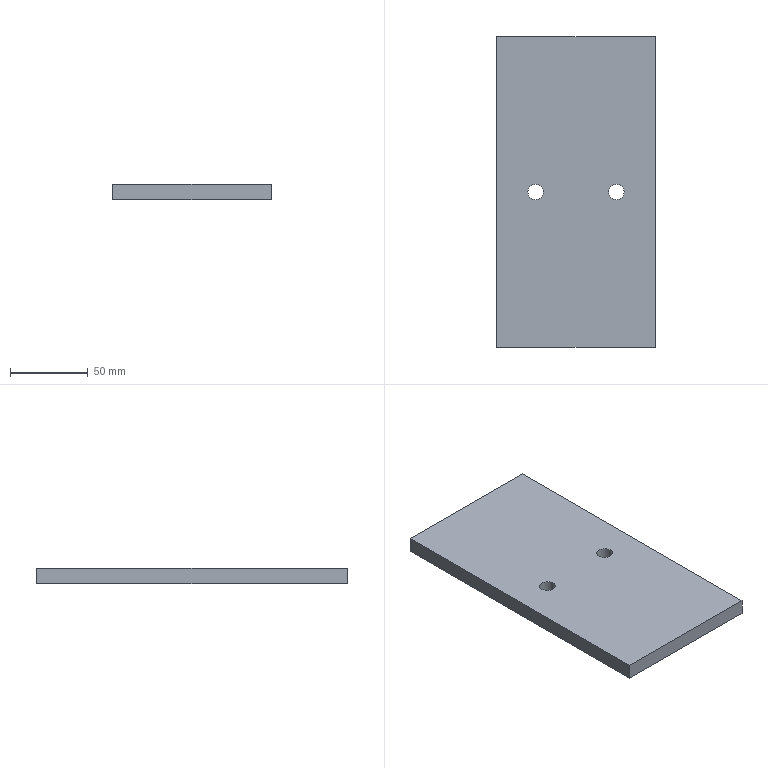Part | STEP file | E3-导轨限位Plate | 1 solid | 10 faces | box 102 x 200 x 10 mm | volume 202429 mm3 | plane 6 | cylinder 4 | commonest cylinder face diameters 10 x4
STEP:
#1=CARTESIAN_POINT('',(0.,0.,0.));
#2=DIRECTION('',(0.,0.,1.));
#3=DIRECTION('',(1.,0.,0.));
#4=AXIS2_PLACEMENT_3D('',#1,#2,#3);
#5=CARTESIAN_POINT('',(-21.,0.,0.));
#6=VERTEX_POINT('',#5);
#7=CARTESIAN_POINT('',(-21.,0.,-10.));
#8=VERTEX_POINT('',#7);
#9=CARTESIAN_POINT('',(-21.,0.,-10.));
#10=DIRECTION('',(0.,0.,-1.));
#11=VECTOR('',#10,1.);
#12=LINE('',#9,#11);
#13=CARTESIAN_POINT('',(-26.,0.,-10.));
#14=DIRECTION('',(0.,0.,-1.));
#15=DIRECTION('',(1.,0.,0.));
#16=AXIS2_PLACEMENT_3D('',#13,#14,#15);
#17=CYLINDRICAL_SURFACE('',#16,5.);
#18=CARTESIAN_POINT('',(6.283,0.));
#19=DIRECTION('',(0.,1.));
#20=VECTOR('',#19,1.);
#21=LINE('',#18,#20);
#22=(GEOMETRIC_REPRESENTATION_CONTEXT(2)PARAMETRIC_REPRESENTATION_CONTEXT()REPRESENTATION_CONTEXT('',''));
#23=DEFINITIONAL_REPRESENTATION('',(#21),#22);
#24=PCURVE('',#17,#23);
#25=CARTESIAN_POINT('',(-26.,0.,-10.));
#26=DIRECTION('',(0.,0.,-1.));
#27=DIRECTION('',(1.,0.,0.));
#28=AXIS2_PLACEMENT_3D('',#25,#26,#27);
#29=CYLINDRICAL_SURFACE('',#28,5.);
#30=CARTESIAN_POINT('',(0.,0.));
#31=DIRECTION('',(0.,1.));
#32=VECTOR('',#31,1.);
#33=LINE('',#30,#32);
#34=(GEOMETRIC_REPRESENTATION_CONTEXT(2)PARAMETRIC_REPRESENTATION_CONTEXT()REPRESENTATION_CONTEXT('',''));
#35=DEFINITIONAL_REPRESENTATION('',(#33),#34);
#36=PCURVE('',#29,#35);
#37=SURFACE_CURVE('',#12,(#24,#36),.PCURVE_S1.);
#38=EDGE_CURVE('',#6,#8,#37,.T.);
#39=ORIENTED_EDGE('',*,*,#38,.T.);
#40=CARTESIAN_POINT('',(-31.,0.,-10.));
#41=VERTEX_POINT('',#40);
#42=CARTESIAN_POINT('',(-26.,0.,-10.));
#43=DIRECTION('',(0.,0.,1.));
#44=DIRECTION('',(1.,0.,0.));
#45=AXIS2_PLACEMENT_3D('',#42,#43,#44);
#46=CIRCLE('',#45,5.);
#47=CARTESIAN_POINT('',(6.283,0.));
#48=DIRECTION('',(-1.,0.));
#49=VECTOR('',#48,1.);
#50=LINE('',#47,#49);
#51=(GEOMETRIC_REPRESENTATION_CONTEXT(2)PARAMETRIC_REPRESENTATION_CONTEXT()REPRESENTATION_CONTEXT('',''));
#52=DEFINITIONAL_REPRESENTATION('',(#50),#51);
#53=PCURVE('',#17,#52);
#54=CARTESIAN_POINT('',(0.,0.,-10.));
#55=DIRECTION('',(0.,0.,-1.));
#56=DIRECTION('',(1.,0.,0.));
#57=AXIS2_PLACEMENT_3D('',#54,#55,#56);
#58=PLANE('',#57);
#59=CARTESIAN_POINT('',(-21.,0.));
#60=CARTESIAN_POINT('',(-21.,-8.66));
#61=CARTESIAN_POINT('',(-28.5,-4.33));
#62=CARTESIAN_POINT('',(-36.,0.));
#63=CARTESIAN_POINT('',(-28.5,4.33));
#64=CARTESIAN_POINT('',(-21.,8.66));
#65=CARTESIAN_POINT('',(-21.,0.));
#66=(BOUNDED_CURVE()B_SPLINE_CURVE(2,(#59,#60,#61,#62,#63,#64,#65),.UNSPECIFIED.,.T.,.F.)B_SPLINE_CURVE_WITH_KNOTS((1,2,2,2,2,1),(-2.094,0.,2.094,4.189,6.283,8.378),.UNSPECIFIED.)CURVE()GEOMETRIC_REPRESENTATION_ITEM()RATIONAL_B_SPLINE_CURVE((1.,0.5,1.,0.5,1.,0.5,1.))REPRESENTATION_ITEM(''));
#67=(GEOMETRIC_REPRESENTATION_CONTEXT(2)PARAMETRIC_REPRESENTATION_CONTEXT()REPRESENTATION_CONTEXT('',''));
#68=DEFINITIONAL_REPRESENTATION('',(#66),#67);
#69=PCURVE('',#58,#68);
#70=SURFACE_CURVE('',#46,(#53,#69),.PCURVE_S1.);
#71=EDGE_CURVE('',#8,#41,#70,.T.);
#72=ORIENTED_EDGE('',*,*,#71,.T.);
#73=CARTESIAN_POINT('',(-31.,0.,0.));
#74=VERTEX_POINT('',#73);
#75=CARTESIAN_POINT('',(-31.,0.,-10.));
#76=DIRECTION('',(0.,0.,-1.));
#77=VECTOR('',#76,1.);
#78=LINE('',#75,#77);
#79=CARTESIAN_POINT('',(3.142,0.));
#80=DIRECTION('',(0.,1.));
#81=VECTOR('',#80,1.);
#82=LINE('',#79,#81);
#83=(GEOMETRIC_REPRESENTATION_CONTEXT(2)PARAMETRIC_REPRESENTATION_CONTEXT()REPRESENTATION_CONTEXT('',''));
#84=DEFINITIONAL_REPRESENTATION('',(#82),#83);
#85=PCURVE('',#17,#84);
#86=CARTESIAN_POINT('',(3.142,0.));
#87=DIRECTION('',(0.,1.));
#88=VECTOR('',#87,1.);
#89=LINE('',#86,#88);
#90=(GEOMETRIC_REPRESENTATION_CONTEXT(2)PARAMETRIC_REPRESENTATION_CONTEXT()REPRESENTATION_CONTEXT('',''));
#91=DEFINITIONAL_REPRESENTATION('',(#89),#90);
#92=PCURVE('',#29,#91);
#93=SURFACE_CURVE('',#78,(#85,#92),.PCURVE_S1.);
#94=EDGE_CURVE('',#74,#41,#93,.T.);
#95=ORIENTED_EDGE('',*,*,#94,.F.);
#96=CARTESIAN_POINT('',(-26.,0.,0.));
#97=DIRECTION('',(0.,0.,1.));
#98=DIRECTION('',(1.,0.,0.));
#99=AXIS2_PLACEMENT_3D('',#96,#97,#98);
#100=CIRCLE('',#99,5.);
#101=CARTESIAN_POINT('',(6.283,-10.));
#102=DIRECTION('',(-1.,0.));
#103=VECTOR('',#102,1.);
#104=LINE('',#101,#103);
#105=(GEOMETRIC_REPRESENTATION_CONTEXT(2)PARAMETRIC_REPRESENTATION_CONTEXT()REPRESENTATION_CONTEXT('',''));
#106=DEFINITIONAL_REPRESENTATION('',(#104),#105);
#107=PCURVE('',#17,#106);
#108=CARTESIAN_POINT('',(0.,0.,0.));
#109=DIRECTION('',(0.,0.,-1.));
#110=DIRECTION('',(1.,0.,0.));
#111=AXIS2_PLACEMENT_3D('',#108,#109,#110);
#112=PLANE('',#111);
#113=CARTESIAN_POINT('',(-21.,0.));
#114=CARTESIAN_POINT('',(-21.,-8.66));
#115=CARTESIAN_POINT('',(-28.5,-4.33));
#116=CARTESIAN_POINT('',(-36.,0.));
#117=CARTESIAN_POINT('',(-28.5,4.33));
#118=CARTESIAN_POINT('',(-21.,8.66));
#119=CARTESIAN_POINT('',(-21.,0.));
#120=(BOUNDED_CURVE()B_SPLINE_CURVE(2,(#113,#114,#115,#116,#117,#118,#119),.UNSPECIFIED.,.T.,.F.)B_SPLINE_CURVE_WITH_KNOTS((1,2,2,2,2,1),(-2.094,0.,2.094,4.189,6.283,8.378),.UNSPECIFIED.)CURVE()GEOMETRIC_REPRESENTATION_ITEM()RATIONAL_B_SPLINE_CURVE((1.,0.5,1.,0.5,1.,0.5,1.))REPRESENTATION_ITEM(''));
#121=(GEOMETRIC_REPRESENTATION_CONTEXT(2)PARAMETRIC_REPRESENTATION_CONTEXT()REPRESENTATION_CONTEXT('',''));
#122=DEFINITIONAL_REPRESENTATION('',(#120),#121);
#123=PCURVE('',#112,#122);
#124=SURFACE_CURVE('',#100,(#107,#123),.PCURVE_S1.);
#125=EDGE_CURVE('',#6,#74,#124,.T.);
#126=ORIENTED_EDGE('',*,*,#125,.F.);
#127=EDGE_LOOP('',(#39,#72,#95,#126));
#128=FACE_BOUND('',#127,.F.);
#129=ADVANCED_FACE('',(#128),#17,.F.);
#130=CARTESIAN_POINT('',(31.,0.,0.));
#131=VERTEX_POINT('',#130);
#132=CARTESIAN_POINT('',(31.,0.,-10.));
#133=VERTEX_POINT('',#132);
#134=CARTESIAN_POINT('',(31.,0.,-10.));
#135=DIRECTION('',(0.,0.,-1.));
#136=VECTOR('',#135,1.);
#137=LINE('',#134,#136);
#138=CARTESIAN_POINT('',(26.,0.,-10.));
#139=DIRECTION('',(0.,0.,-1.));
#140=DIRECTION('',(1.,0.,0.));
#141=AXIS2_PLACEMENT_3D('',#138,#139,#140);
#142=CYLINDRICAL_SURFACE('',#141,5.);
#143=CARTESIAN_POINT('',(6.283,0.));
#144=DIRECTION('',(0.,1.));
#145=VECTOR('',#144,1.);
#146=LINE('',#143,#145);
#147=(GEOMETRIC_REPRESENTATION_CONTEXT(2)PARAMETRIC_REPRESENTATION_CONTEXT()REPRESENTATION_CONTEXT('',''));
#148=DEFINITIONAL_REPRESENTATION('',(#146),#147);
#149=PCURVE('',#142,#148);
#150=CARTESIAN_POINT('',(26.,0.,-10.));
#151=DIRECTION('',(0.,0.,-1.));
#152=DIRECTION('',(1.,0.,0.));
#153=AXIS2_PLACEMENT_3D('',#150,#151,#152);
#154=CYLINDRICAL_SURFACE('',#153,5.);
#155=CARTESIAN_POINT('',(0.,0.));
#156=DIRECTION('',(0.,1.));
#157=VECTOR('',#156,1.);
#158=LINE('',#155,#157);
#159=(GEOMETRIC_REPRESENTATION_CONTEXT(2)PARAMETRIC_REPRESENTATION_CONTEXT()REPRESENTATION_CONTEXT('',''));
#160=DEFINITIONAL_REPRESENTATION('',(#158),#159);
#161=PCURVE('',#154,#160);
#162=SURFACE_CURVE('',#137,(#149,#161),.PCURVE_S1.);
#163=EDGE_CURVE('',#131,#133,#162,.T.);
#164=ORIENTED_EDGE('',*,*,#163,.T.);
#165=CARTESIAN_POINT('',(21.,0.,-10.));
#166=VERTEX_POINT('',#165);
#167=CARTESIAN_POINT('',(26.,0.,-10.));
#168=DIRECTION('',(0.,0.,1.));
#169=DIRECTION('',(1.,0.,0.));
#170=AXIS2_PLACEMENT_3D('',#167,#168,#169);
#171=CIRCLE('',#170,5.);
#172=CARTESIAN_POINT('',(6.283,0.));
#173=DIRECTION('',(-1.,0.));
#174=VECTOR('',#173,1.);
#175=LINE('',#172,#174);
#176=(GEOMETRIC_REPRESENTATION_CONTEXT(2)PARAMETRIC_REPRESENTATION_CONTEXT()REPRESENTATION_CONTEXT('',''));
#177=DEFINITIONAL_REPRESENTATION('',(#175),#176);
#178=PCURVE('',#142,#177);
#179=CARTESIAN_POINT('',(31.,0.));
#180=CARTESIAN_POINT('',(31.,-8.66));
#181=CARTESIAN_POINT('',(23.5,-4.33));
#182=CARTESIAN_POINT('',(16.,0.));
#183=CARTESIAN_POINT('',(23.5,4.33));
#184=CARTESIAN_POINT('',(31.,8.66));
#185=CARTESIAN_POINT('',(31.,0.));
#186=(BOUNDED_CURVE()B_SPLINE_CURVE(2,(#179,#180,#181,#182,#183,#184,#185),.UNSPECIFIED.,.T.,.F.)B_SPLINE_CURVE_WITH_KNOTS((1,2,2,2,2,1),(-2.094,0.,2.094,4.189,6.283,8.378),.UNSPECIFIED.)CURVE()GEOMETRIC_REPRESENTATION_ITEM()RATIONAL_B_SPLINE_CURVE((1.,0.5,1.,0.5,1.,0.5,1.))REPRESENTATION_ITEM(''));
#187=(GEOMETRIC_REPRESENTATION_CONTEXT(2)PARAMETRIC_REPRESENTATION_CONTEXT()REPRESENTATION_CONTEXT('',''));
#188=DEFINITIONAL_REPRESENTATION('',(#186),#187);
#189=PCURVE('',#58,#188);
#190=SURFACE_CURVE('',#171,(#178,#189),.PCURVE_S1.);
#191=EDGE_CURVE('',#133,#166,#190,.T.);
#192=ORIENTED_EDGE('',*,*,#191,.T.);
#193=CARTESIAN_POINT('',(21.,0.,0.));
#194=VERTEX_POINT('',#193);
#195=CARTESIAN_POINT('',(21.,0.,-10.));
#196=DIRECTION('',(0.,0.,-1.));
#197=VECTOR('',#196,1.);
#198=LINE('',#195,#197);
#199=CARTESIAN_POINT('',(3.142,0.));
#200=DIRECTION('',(0.,1.));
#201=VECTOR('',#200,1.);
#202=LINE('',#199,#201);
#203=(GEOMETRIC_REPRESENTATION_CONTEXT(2)PARAMETRIC_REPRESENTATION_CONTEXT()REPRESENTATION_CONTEXT('',''));
#204=DEFINITIONAL_REPRESENTATION('',(#202),#203);
#205=PCURVE('',#142,#204);
#206=CARTESIAN_POINT('',(3.142,0.));
#207=DIRECTION('',(0.,1.));
#208=VECTOR('',#207,1.);
#209=LINE('',#206,#208);
#210=(GEOMETRIC_REPRESENTATION_CONTEXT(2)PARAMETRIC_REPRESENTATION_CONTEXT()REPRESENTATION_CONTEXT('',''));
#211=DEFINITIONAL_REPRESENTATION('',(#209),#210);
#212=PCURVE('',#154,#211);
#213=SURFACE_CURVE('',#198,(#205,#212),.PCURVE_S1.);
#214=EDGE_CURVE('',#194,#166,#213,.T.);
#215=ORIENTED_EDGE('',*,*,#214,.F.);
#216=CARTESIAN_POINT('',(26.,0.,0.));
#217=DIRECTION('',(0.,0.,1.));
#218=DIRECTION('',(1.,0.,0.));
#219=AXIS2_PLACEMENT_3D('',#216,#217,#218);
#220=CIRCLE('',#219,5.);
#221=CARTESIAN_POINT('',(6.283,-10.));
#222=DIRECTION('',(-1.,0.));
#223=VECTOR('',#222,1.);
#224=LINE('',#221,#223);
#225=(GEOMETRIC_REPRESENTATION_CONTEXT(2)PARAMETRIC_REPRESENTATION_CONTEXT()REPRESENTATION_CONTEXT('',''));
#226=DEFINITIONAL_REPRESENTATION('',(#224),#225);
#227=PCURVE('',#142,#226);
#228=CARTESIAN_POINT('',(31.,0.));
#229=CARTESIAN_POINT('',(31.,-8.66));
#230=CARTESIAN_POINT('',(23.5,-4.33));
#231=CARTESIAN_POINT('',(16.,0.));
#232=CARTESIAN_POINT('',(23.5,4.33));
#233=CARTESIAN_POINT('',(31.,8.66));
#234=CARTESIAN_POINT('',(31.,0.));
#235=(BOUNDED_CURVE()B_SPLINE_CURVE(2,(#228,#229,#230,#231,#232,#233,#234),.UNSPECIFIED.,.T.,.F.)B_SPLINE_CURVE_WITH_KNOTS((1,2,2,2,2,1),(-2.094,0.,2.094,4.189,6.283,8.378),.UNSPECIFIED.)CURVE()GEOMETRIC_REPRESENTATION_ITEM()RATIONAL_B_SPLINE_CURVE((1.,0.5,1.,0.5,1.,0.5,1.))REPRESENTATION_ITEM(''));
#236=(GEOMETRIC_REPRESENTATION_CONTEXT(2)PARAMETRIC_REPRESENTATION_CONTEXT()REPRESENTATION_CONTEXT('',''));
#237=DEFINITIONAL_REPRESENTATION('',(#235),#236);
#238=PCURVE('',#112,#237);
#239=SURFACE_CURVE('',#220,(#227,#238),.PCURVE_S1.);
#240=EDGE_CURVE('',#131,#194,#239,.T.);
#241=ORIENTED_EDGE('',*,*,#240,.F.);
#242=EDGE_LOOP('',(#164,#192,#215,#241));
#243=FACE_BOUND('',#242,.F.);
#244=ADVANCED_FACE('',(#243),#142,.F.);
#245=CARTESIAN_POINT('',(51.,-100.,0.));
#246=VERTEX_POINT('',#245);
#247=CARTESIAN_POINT('',(51.,100.,0.));
#248=VERTEX_POINT('',#247);
#249=CARTESIAN_POINT('',(51.,100.,0.));
#250=DIRECTION('',(0.,1.,0.));
#251=VECTOR('',#250,1.);
#252=LINE('',#249,#251);
#253=CARTESIAN_POINT('',(51.,100.,-10.));
#254=DIRECTION('',(-1.,0.,0.));
#255=DIRECTION('',(0.,-1.,0.));
#256=AXIS2_PLACEMENT_3D('',#253,#254,#255);
#257=PLANE('',#256);
#258=CARTESIAN_POINT('',(0.,10.));
#259=DIRECTION('',(-1.,0.));
#260=VECTOR('',#259,1.);
#261=LINE('',#258,#260);
#262=(GEOMETRIC_REPRESENTATION_CONTEXT(2)PARAMETRIC_REPRESENTATION_CONTEXT()REPRESENTATION_CONTEXT('',''));
#263=DEFINITIONAL_REPRESENTATION('',(#261),#262);
#264=PCURVE('',#257,#263);
#265=CARTESIAN_POINT('',(51.,-100.));
#266=DIRECTION('',(0.,-1.));
#267=VECTOR('',#266,1.);
#268=LINE('',#265,#267);
#269=(GEOMETRIC_REPRESENTATION_CONTEXT(2)PARAMETRIC_REPRESENTATION_CONTEXT()REPRESENTATION_CONTEXT('',''));
#270=DEFINITIONAL_REPRESENTATION('',(#268),#269);
#271=PCURVE('',#112,#270);
#272=SURFACE_CURVE('',#252,(#264,#271),.PCURVE_S1.);
#273=EDGE_CURVE('',#246,#248,#272,.T.);
#274=ORIENTED_EDGE('',*,*,#273,.F.);
#275=CARTESIAN_POINT('',(51.,-100.,-10.));
#276=VERTEX_POINT('',#275);
#277=CARTESIAN_POINT('',(51.,-100.,-10.));
#278=DIRECTION('',(0.,0.,1.));
#279=VECTOR('',#278,1.);
#280=LINE('',#277,#279);
#281=CARTESIAN_POINT('',(200.,0.));
#282=DIRECTION('',(0.,1.));
#283=VECTOR('',#282,1.);
#284=LINE('',#281,#283);
#285=(GEOMETRIC_REPRESENTATION_CONTEXT(2)PARAMETRIC_REPRESENTATION_CONTEXT()REPRESENTATION_CONTEXT('',''));
#286=DEFINITIONAL_REPRESENTATION('',(#284),#285);
#287=PCURVE('',#257,#286);
#288=CARTESIAN_POINT('',(-51.,-100.,-10.));
#289=DIRECTION('',(0.,1.,0.));
#290=DIRECTION('',(0.,0.,-1.));
#291=AXIS2_PLACEMENT_3D('',#288,#289,#290);
#292=PLANE('',#291);
#293=CARTESIAN_POINT('',(0.,-102.));
#294=DIRECTION('',(-1.,0.));
#295=VECTOR('',#294,1.);
#296=LINE('',#293,#295);
#297=(GEOMETRIC_REPRESENTATION_CONTEXT(2)PARAMETRIC_REPRESENTATION_CONTEXT()REPRESENTATION_CONTEXT('',''));
#298=DEFINITIONAL_REPRESENTATION('',(#296),#297);
#299=PCURVE('',#292,#298);
#300=SURFACE_CURVE('',#280,(#287,#299),.PCURVE_S1.);
#301=EDGE_CURVE('',#276,#246,#300,.T.);
#302=ORIENTED_EDGE('',*,*,#301,.F.);
#303=CARTESIAN_POINT('',(51.,100.,-10.));
#304=VERTEX_POINT('',#303);
#305=CARTESIAN_POINT('',(51.,100.,-10.));
#306=DIRECTION('',(0.,1.,0.));
#307=VECTOR('',#306,1.);
#308=LINE('',#305,#307);
#309=CARTESIAN_POINT('',(0.,0.));
#310=DIRECTION('',(-1.,0.));
#311=VECTOR('',#310,1.);
#312=LINE('',#309,#311);
#313=(GEOMETRIC_REPRESENTATION_CONTEXT(2)PARAMETRIC_REPRESENTATION_CONTEXT()REPRESENTATION_CONTEXT('',''));
#314=DEFINITIONAL_REPRESENTATION('',(#312),#313);
#315=PCURVE('',#257,#314);
#316=CARTESIAN_POINT('',(51.,-100.));
#317=DIRECTION('',(0.,-1.));
#318=VECTOR('',#317,1.);
#319=LINE('',#316,#318);
#320=(GEOMETRIC_REPRESENTATION_CONTEXT(2)PARAMETRIC_REPRESENTATION_CONTEXT()REPRESENTATION_CONTEXT('',''));
#321=DEFINITIONAL_REPRESENTATION('',(#319),#320);
#322=PCURVE('',#58,#321);
#323=SURFACE_CURVE('',#308,(#315,#322),.PCURVE_S1.);
#324=EDGE_CURVE('',#276,#304,#323,.T.);
#325=ORIENTED_EDGE('',*,*,#324,.T.);
#326=CARTESIAN_POINT('',(51.,100.,-10.));
#327=DIRECTION('',(0.,0.,1.));
#328=VECTOR('',#327,1.);
#329=LINE('',#326,#328);
#330=CARTESIAN_POINT('',(0.,0.));
#331=DIRECTION('',(0.,1.));
#332=VECTOR('',#331,1.);
#333=LINE('',#330,#332);
#334=(GEOMETRIC_REPRESENTATION_CONTEXT(2)PARAMETRIC_REPRESENTATION_CONTEXT()REPRESENTATION_CONTEXT('',''));
#335=DEFINITIONAL_REPRESENTATION('',(#333),#334);
#336=PCURVE('',#257,#335);
#337=CARTESIAN_POINT('',(-51.,100.,-10.));
#338=DIRECTION('',(0.,-1.,0.));
#339=DIRECTION('',(0.,0.,1.));
#340=AXIS2_PLACEMENT_3D('',#337,#338,#339);
#341=PLANE('',#340);
#342=CARTESIAN_POINT('',(0.,-102.));
#343=DIRECTION('',(1.,0.));
#344=VECTOR('',#343,1.);
#345=LINE('',#342,#344);
#346=(GEOMETRIC_REPRESENTATION_CONTEXT(2)PARAMETRIC_REPRESENTATION_CONTEXT()REPRESENTATION_CONTEXT('',''));
#347=DEFINITIONAL_REPRESENTATION('',(#345),#346);
#348=PCURVE('',#341,#347);
#349=SURFACE_CURVE('',#329,(#336,#348),.PCURVE_S1.);
#350=EDGE_CURVE('',#304,#248,#349,.T.);
#351=ORIENTED_EDGE('',*,*,#350,.T.);
#352=EDGE_LOOP('',(#274,#302,#325,#351));
#353=FACE_BOUND('',#352,.T.);
#354=ADVANCED_FACE('',(#353),#257,.F.);
#355=CARTESIAN_POINT('',(-51.,100.,0.));
#356=VERTEX_POINT('',#355);
#357=CARTESIAN_POINT('',(-51.,100.,0.));
#358=DIRECTION('',(-1.,0.,0.));
#359=VECTOR('',#358,1.);
#360=LINE('',#357,#359);
#361=CARTESIAN_POINT('',(10.,0.));
#362=DIRECTION('',(0.,1.));
#363=VECTOR('',#362,1.);
#364=LINE('',#361,#363);
#365=(GEOMETRIC_REPRESENTATION_CONTEXT(2)PARAMETRIC_REPRESENTATION_CONTEXT()REPRESENTATION_CONTEXT('',''));
#366=DEFINITIONAL_REPRESENTATION('',(#364),#365);
#367=PCURVE('',#341,#366);
#368=CARTESIAN_POINT('',(-51.,-100.));
#369=DIRECTION('',(-1.,0.));
#370=VECTOR('',#369,1.);
#371=LINE('',#368,#370);
#372=(GEOMETRIC_REPRESENTATION_CONTEXT(2)PARAMETRIC_REPRESENTATION_CONTEXT()REPRESENTATION_CONTEXT('',''));
#373=DEFINITIONAL_REPRESENTATION('',(#371),#372);
#374=PCURVE('',#112,#373);
#375=SURFACE_CURVE('',#360,(#367,#374),.PCURVE_S1.);
#376=EDGE_CURVE('',#248,#356,#375,.T.);
#377=ORIENTED_EDGE('',*,*,#376,.F.);
#378=ORIENTED_EDGE('',*,*,#350,.F.);
#379=CARTESIAN_POINT('',(-51.,100.,-10.));
#380=VERTEX_POINT('',#379);
#381=CARTESIAN_POINT('',(-51.,100.,-10.));
#382=DIRECTION('',(-1.,0.,0.));
#383=VECTOR('',#382,1.);
#384=LINE('',#381,#383);
#385=CARTESIAN_POINT('',(0.,0.));
#386=DIRECTION('',(0.,1.));
#387=VECTOR('',#386,1.);
#388=LINE('',#385,#387);
#389=(GEOMETRIC_REPRESENTATION_CONTEXT(2)PARAMETRIC_REPRESENTATION_CONTEXT()REPRESENTATION_CONTEXT('',''));
#390=DEFINITIONAL_REPRESENTATION('',(#388),#389);
#391=PCURVE('',#341,#390);
#392=CARTESIAN_POINT('',(-51.,-100.));
#393=DIRECTION('',(-1.,0.));
#394=VECTOR('',#393,1.);
#395=LINE('',#392,#394);
#396=(GEOMETRIC_REPRESENTATION_CONTEXT(2)PARAMETRIC_REPRESENTATION_CONTEXT()REPRESENTATION_CONTEXT('',''));
#397=DEFINITIONAL_REPRESENTATION('',(#395),#396);
#398=PCURVE('',#58,#397);
#399=SURFACE_CURVE('',#384,(#391,#398),.PCURVE_S1.);
#400=EDGE_CURVE('',#304,#380,#399,.T.);
#401=ORIENTED_EDGE('',*,*,#400,.T.);
#402=CARTESIAN_POINT('',(-51.,100.,-10.));
#403=DIRECTION('',(0.,0.,1.));
#404=VECTOR('',#403,1.);
#405=LINE('',#402,#404);
#406=CARTESIAN_POINT('',(0.,0.));
#407=DIRECTION('',(1.,0.));
#408=VECTOR('',#407,1.);
#409=LINE('',#406,#408);
#410=(GEOMETRIC_REPRESENTATION_CONTEXT(2)PARAMETRIC_REPRESENTATION_CONTEXT()REPRESENTATION_CONTEXT('',''));
#411=DEFINITIONAL_REPRESENTATION('',(#409),#410);
#412=PCURVE('',#341,#411);
#413=CARTESIAN_POINT('',(-51.,100.,-10.));
#414=DIRECTION('',(1.,0.,0.));
#415=DIRECTION('',(0.,1.,0.));
#416=AXIS2_PLACEMENT_3D('',#413,#414,#415);
#417=PLANE('',#416);
#418=CARTESIAN_POINT('',(0.,0.));
#419=DIRECTION('',(0.,1.));
#420=VECTOR('',#419,1.);
#421=LINE('',#418,#420);
#422=(GEOMETRIC_REPRESENTATION_CONTEXT(2)PARAMETRIC_REPRESENTATION_CONTEXT()REPRESENTATION_CONTEXT('',''));
#423=DEFINITIONAL_REPRESENTATION('',(#421),#422);
#424=PCURVE('',#417,#423);
#425=SURFACE_CURVE('',#405,(#412,#424),.PCURVE_S1.);
#426=EDGE_CURVE('',#380,#356,#425,.T.);
#427=ORIENTED_EDGE('',*,*,#426,.T.);
#428=EDGE_LOOP('',(#377,#378,#401,#427));
#429=FACE_BOUND('',#428,.T.);
#430=ADVANCED_FACE('',(#429),#341,.F.);
#431=CARTESIAN_POINT('',(-51.,-100.,0.));
#432=VERTEX_POINT('',#431);
#433=CARTESIAN_POINT('',(-51.,100.,0.));
#434=DIRECTION('',(0.,-1.,0.));
#435=VECTOR('',#434,1.);
#436=LINE('',#433,#435);
#437=CARTESIAN_POINT('',(0.,10.));
#438=DIRECTION('',(-1.,0.));
#439=VECTOR('',#438,1.);
#440=LINE('',#437,#439);
#441=(GEOMETRIC_REPRESENTATION_CONTEXT(2)PARAMETRIC_REPRESENTATION_CONTEXT()REPRESENTATION_CONTEXT('',''));
#442=DEFINITIONAL_REPRESENTATION('',(#440),#441);
#443=PCURVE('',#417,#442);
#444=CARTESIAN_POINT('',(-51.,-100.));
#445=DIRECTION('',(0.,1.));
#446=VECTOR('',#445,1.);
#447=LINE('',#444,#446);
#448=(GEOMETRIC_REPRESENTATION_CONTEXT(2)PARAMETRIC_REPRESENTATION_CONTEXT()REPRESENTATION_CONTEXT('',''));
#449=DEFINITIONAL_REPRESENTATION('',(#447),#448);
#450=PCURVE('',#112,#449);
#451=SURFACE_CURVE('',#436,(#443,#450),.PCURVE_S1.);
#452=EDGE_CURVE('',#356,#432,#451,.T.);
#453=ORIENTED_EDGE('',*,*,#452,.F.);
#454=ORIENTED_EDGE('',*,*,#426,.F.);
#455=CARTESIAN_POINT('',(-51.,-100.,-10.));
#456=VERTEX_POINT('',#455);
#457=CARTESIAN_POINT('',(-51.,100.,-10.));
#458=DIRECTION('',(0.,-1.,0.));
#459=VECTOR('',#458,1.);
#460=LINE('',#457,#459);
#461=CARTESIAN_POINT('',(0.,0.));
#462=DIRECTION('',(-1.,0.));
#463=VECTOR('',#462,1.);
#464=LINE('',#461,#463);
#465=(GEOMETRIC_REPRESENTATION_CONTEXT(2)PARAMETRIC_REPRESENTATION_CONTEXT()REPRESENTATION_CONTEXT('',''));
#466=DEFINITIONAL_REPRESENTATION('',(#464),#465);
#467=PCURVE('',#417,#466);
#468=CARTESIAN_POINT('',(-51.,-100.));
#469=DIRECTION('',(0.,1.));
#470=VECTOR('',#469,1.);
#471=LINE('',#468,#470);
#472=(GEOMETRIC_REPRESENTATION_CONTEXT(2)PARAMETRIC_REPRESENTATION_CONTEXT()REPRESENTATION_CONTEXT('',''));
#473=DEFINITIONAL_REPRESENTATION('',(#471),#472);
#474=PCURVE('',#58,#473);
#475=SURFACE_CURVE('',#460,(#467,#474),.PCURVE_S1.);
#476=EDGE_CURVE('',#380,#456,#475,.T.);
#477=ORIENTED_EDGE('',*,*,#476,.T.);
#478=CARTESIAN_POINT('',(-51.,-100.,-10.));
#479=DIRECTION('',(0.,0.,1.));
#480=VECTOR('',#479,1.);
#481=LINE('',#478,#480);
#482=CARTESIAN_POINT('',(-200.,0.));
#483=DIRECTION('',(0.,1.));
#484=VECTOR('',#483,1.);
#485=LINE('',#482,#484);
#486=(GEOMETRIC_REPRESENTATION_CONTEXT(2)PARAMETRIC_REPRESENTATION_CONTEXT()REPRESENTATION_CONTEXT('',''));
#487=DEFINITIONAL_REPRESENTATION('',(#485),#486);
#488=PCURVE('',#417,#487);
#489=CARTESIAN_POINT('',(0.,0.));
#490=DIRECTION('',(-1.,0.));
#491=VECTOR('',#490,1.);
#492=LINE('',#489,#491);
#493=(GEOMETRIC_REPRESENTATION_CONTEXT(2)PARAMETRIC_REPRESENTATION_CONTEXT()REPRESENTATION_CONTEXT('',''));
#494=DEFINITIONAL_REPRESENTATION('',(#492),#493);
#495=PCURVE('',#292,#494);
#496=SURFACE_CURVE('',#481,(#488,#495),.PCURVE_S1.);
#497=EDGE_CURVE('',#456,#432,#496,.T.);
#498=ORIENTED_EDGE('',*,*,#497,.T.);
#499=EDGE_LOOP('',(#453,#454,#477,#498));
#500=FACE_BOUND('',#499,.T.);
#501=ADVANCED_FACE('',(#500),#417,.F.);
#502=CARTESIAN_POINT('',(-51.,-100.,0.));
#503=DIRECTION('',(1.,0.,0.));
#504=VECTOR('',#503,1.);
#505=LINE('',#502,#504);
#506=CARTESIAN_POINT('',(-10.,0.));
#507=DIRECTION('',(0.,-1.));
#508=VECTOR('',#507,1.);
#509=LINE('',#506,#508);
#510=(GEOMETRIC_REPRESENTATION_CONTEXT(2)PARAMETRIC_REPRESENTATION_CONTEXT()REPRESENTATION_CONTEXT('',''));
#511=DEFINITIONAL_REPRESENTATION('',(#509),#510);
#512=PCURVE('',#292,#511);
#513=CARTESIAN_POINT('',(-51.,100.));
#514=DIRECTION('',(1.,0.));
#515=VECTOR('',#514,1.);
#516=LINE('',#513,#515);
#517=(GEOMETRIC_REPRESENTATION_CONTEXT(2)PARAMETRIC_REPRESENTATION_CONTEXT()REPRESENTATION_CONTEXT('',''));
#518=DEFINITIONAL_REPRESENTATION('',(#516),#517);
#519=PCURVE('',#112,#518);
#520=SURFACE_CURVE('',#505,(#512,#519),.PCURVE_S1.);
#521=EDGE_CURVE('',#432,#246,#520,.T.);
#522=ORIENTED_EDGE('',*,*,#521,.F.);
#523=ORIENTED_EDGE('',*,*,#497,.F.);
#524=CARTESIAN_POINT('',(-51.,-100.,-10.));
#525=DIRECTION('',(1.,0.,0.));
#526=VECTOR('',#525,1.);
#527=LINE('',#524,#526);
#528=CARTESIAN_POINT('',(0.,0.));
#529=DIRECTION('',(0.,-1.));
#530=VECTOR('',#529,1.);
#531=LINE('',#528,#530);
#532=(GEOMETRIC_REPRESENTATION_CONTEXT(2)PARAMETRIC_REPRESENTATION_CONTEXT()REPRESENTATION_CONTEXT('',''));
#533=DEFINITIONAL_REPRESENTATION('',(#531),#532);
#534=PCURVE('',#292,#533);
#535=CARTESIAN_POINT('',(-51.,100.));
#536=DIRECTION('',(1.,0.));
#537=VECTOR('',#536,1.);
#538=LINE('',#535,#537);
#539=(GEOMETRIC_REPRESENTATION_CONTEXT(2)PARAMETRIC_REPRESENTATION_CONTEXT()REPRESENTATION_CONTEXT('',''));
#540=DEFINITIONAL_REPRESENTATION('',(#538),#539);
#541=PCURVE('',#58,#540);
#542=SURFACE_CURVE('',#527,(#534,#541),.PCURVE_S1.);
#543=EDGE_CURVE('',#456,#276,#542,.T.);
#544=ORIENTED_EDGE('',*,*,#543,.T.);
#545=ORIENTED_EDGE('',*,*,#301,.T.);
#546=EDGE_LOOP('',(#522,#523,#544,#545));
#547=FACE_BOUND('',#546,.T.);
#548=ADVANCED_FACE('',(#547),#292,.F.);
#549=ORIENTED_EDGE('',*,*,#71,.T.);
#550=CARTESIAN_POINT('',(-26.,0.,-10.));
#551=DIRECTION('',(0.,0.,1.));
#552=DIRECTION('',(1.,0.,0.));
#553=AXIS2_PLACEMENT_3D('',#550,#551,#552);
#554=CIRCLE('',#553,5.);
#555=CARTESIAN_POINT('',(-21.,0.));
#556=CARTESIAN_POINT('',(-21.,-8.66));
#557=CARTESIAN_POINT('',(-28.5,-4.33));
#558=CARTESIAN_POINT('',(-36.,0.));
#559=CARTESIAN_POINT('',(-28.5,4.33));
#560=CARTESIAN_POINT('',(-21.,8.66));
#561=CARTESIAN_POINT('',(-21.,0.));
#562=(BOUNDED_CURVE()B_SPLINE_CURVE(2,(#555,#556,#557,#558,#559,#560,#561),.UNSPECIFIED.,.T.,.F.)B_SPLINE_CURVE_WITH_KNOTS((1,2,2,2,2,1),(-2.094,0.,2.094,4.189,6.283,8.378),.UNSPECIFIED.)CURVE()GEOMETRIC_REPRESENTATION_ITEM()RATIONAL_B_SPLINE_CURVE((1.,0.5,1.,0.5,1.,0.5,1.))REPRESENTATION_ITEM(''));
#563=(GEOMETRIC_REPRESENTATION_CONTEXT(2)PARAMETRIC_REPRESENTATION_CONTEXT()REPRESENTATION_CONTEXT('',''));
#564=DEFINITIONAL_REPRESENTATION('',(#562),#563);
#565=PCURVE('',#58,#564);
#566=CARTESIAN_POINT('',(6.283,0.));
#567=DIRECTION('',(-1.,0.));
#568=VECTOR('',#567,1.);
#569=LINE('',#566,#568);
#570=(GEOMETRIC_REPRESENTATION_CONTEXT(2)PARAMETRIC_REPRESENTATION_CONTEXT()REPRESENTATION_CONTEXT('',''));
#571=DEFINITIONAL_REPRESENTATION('',(#569),#570);
#572=PCURVE('',#29,#571);
#573=SURFACE_CURVE('',#554,(#565,#572),.PCURVE_S1.);
#574=EDGE_CURVE('',#41,#8,#573,.T.);
#575=ORIENTED_EDGE('',*,*,#574,.T.);
#576=EDGE_LOOP('',(#549,#575));
#577=FACE_BOUND('',#576,.T.);
#578=ORIENTED_EDGE('',*,*,#191,.T.);
#579=CARTESIAN_POINT('',(26.,0.,-10.));
#580=DIRECTION('',(0.,0.,1.));
#581=DIRECTION('',(1.,0.,0.));
#582=AXIS2_PLACEMENT_3D('',#579,#580,#581);
#583=CIRCLE('',#582,5.);
#584=CARTESIAN_POINT('',(31.,0.));
#585=CARTESIAN_POINT('',(31.,-8.66));
#586=CARTESIAN_POINT('',(23.5,-4.33));
#587=CARTESIAN_POINT('',(16.,0.));
#588=CARTESIAN_POINT('',(23.5,4.33));
#589=CARTESIAN_POINT('',(31.,8.66));
#590=CARTESIAN_POINT('',(31.,0.));
#591=(BOUNDED_CURVE()B_SPLINE_CURVE(2,(#584,#585,#586,#587,#588,#589,#590),.UNSPECIFIED.,.T.,.F.)B_SPLINE_CURVE_WITH_KNOTS((1,2,2,2,2,1),(-2.094,0.,2.094,4.189,6.283,8.378),.UNSPECIFIED.)CURVE()GEOMETRIC_REPRESENTATION_ITEM()RATIONAL_B_SPLINE_CURVE((1.,0.5,1.,0.5,1.,0.5,1.))REPRESENTATION_ITEM(''));
#592=(GEOMETRIC_REPRESENTATION_CONTEXT(2)PARAMETRIC_REPRESENTATION_CONTEXT()REPRESENTATION_CONTEXT('',''));
#593=DEFINITIONAL_REPRESENTATION('',(#591),#592);
#594=PCURVE('',#58,#593);
#595=CARTESIAN_POINT('',(6.283,0.));
#596=DIRECTION('',(-1.,0.));
#597=VECTOR('',#596,1.);
#598=LINE('',#595,#597);
#599=(GEOMETRIC_REPRESENTATION_CONTEXT(2)PARAMETRIC_REPRESENTATION_CONTEXT()REPRESENTATION_CONTEXT('',''));
#600=DEFINITIONAL_REPRESENTATION('',(#598),#599);
#601=PCURVE('',#154,#600);
#602=SURFACE_CURVE('',#583,(#594,#601),.PCURVE_S1.);
#603=EDGE_CURVE('',#166,#133,#602,.T.);
#604=ORIENTED_EDGE('',*,*,#603,.T.);
#605=EDGE_LOOP('',(#578,#604));
#606=FACE_BOUND('',#605,.T.);
#607=ORIENTED_EDGE('',*,*,#324,.F.);
#608=ORIENTED_EDGE('',*,*,#543,.F.);
#609=ORIENTED_EDGE('',*,*,#476,.F.);
#610=ORIENTED_EDGE('',*,*,#400,.F.);
#611=EDGE_LOOP('',(#607,#608,#609,#610));
#612=FACE_BOUND('',#611,.T.);
#613=ADVANCED_FACE('',(#577,#606,#612),#58,.T.);
#614=ORIENTED_EDGE('',*,*,#125,.F.);
#615=CARTESIAN_POINT('',(-26.,0.,0.));
#616=DIRECTION('',(0.,0.,1.));
#617=DIRECTION('',(1.,0.,0.));
#618=AXIS2_PLACEMENT_3D('',#615,#616,#617);
#619=CIRCLE('',#618,5.);
#620=CARTESIAN_POINT('',(-21.,0.));
#621=CARTESIAN_POINT('',(-21.,-8.66));
#622=CARTESIAN_POINT('',(-28.5,-4.33));
#623=CARTESIAN_POINT('',(-36.,0.));
#624=CARTESIAN_POINT('',(-28.5,4.33));
#625=CARTESIAN_POINT('',(-21.,8.66));
#626=CARTESIAN_POINT('',(-21.,0.));
#627=(BOUNDED_CURVE()B_SPLINE_CURVE(2,(#620,#621,#622,#623,#624,#625,#626),.UNSPECIFIED.,.T.,.F.)B_SPLINE_CURVE_WITH_KNOTS((1,2,2,2,2,1),(-2.094,0.,2.094,4.189,6.283,8.378),.UNSPECIFIED.)CURVE()GEOMETRIC_REPRESENTATION_ITEM()RATIONAL_B_SPLINE_CURVE((1.,0.5,1.,0.5,1.,0.5,1.))REPRESENTATION_ITEM(''));
#628=(GEOMETRIC_REPRESENTATION_CONTEXT(2)PARAMETRIC_REPRESENTATION_CONTEXT()REPRESENTATION_CONTEXT('',''));
#629=DEFINITIONAL_REPRESENTATION('',(#627),#628);
#630=PCURVE('',#112,#629);
#631=CARTESIAN_POINT('',(6.283,-10.));
#632=DIRECTION('',(-1.,0.));
#633=VECTOR('',#632,1.);
#634=LINE('',#631,#633);
#635=(GEOMETRIC_REPRESENTATION_CONTEXT(2)PARAMETRIC_REPRESENTATION_CONTEXT()REPRESENTATION_CONTEXT('',''));
#636=DEFINITIONAL_REPRESENTATION('',(#634),#635);
#637=PCURVE('',#29,#636);
#638=SURFACE_CURVE('',#619,(#630,#637),.PCURVE_S1.);
#639=EDGE_CURVE('',#74,#6,#638,.T.);
#640=ORIENTED_EDGE('',*,*,#639,.F.);
#641=EDGE_LOOP('',(#614,#640));
#642=FACE_BOUND('',#641,.T.);
#643=ORIENTED_EDGE('',*,*,#240,.F.);
#644=CARTESIAN_POINT('',(26.,0.,0.));
#645=DIRECTION('',(0.,0.,1.));
#646=DIRECTION('',(1.,0.,0.));
#647=AXIS2_PLACEMENT_3D('',#644,#645,#646);
#648=CIRCLE('',#647,5.);
#649=CARTESIAN_POINT('',(31.,0.));
#650=CARTESIAN_POINT('',(31.,-8.66));
#651=CARTESIAN_POINT('',(23.5,-4.33));
#652=CARTESIAN_POINT('',(16.,0.));
#653=CARTESIAN_POINT('',(23.5,4.33));
#654=CARTESIAN_POINT('',(31.,8.66));
#655=CARTESIAN_POINT('',(31.,0.));
#656=(BOUNDED_CURVE()B_SPLINE_CURVE(2,(#649,#650,#651,#652,#653,#654,#655),.UNSPECIFIED.,.T.,.F.)B_SPLINE_CURVE_WITH_KNOTS((1,2,2,2,2,1),(-2.094,0.,2.094,4.189,6.283,8.378),.UNSPECIFIED.)CURVE()GEOMETRIC_REPRESENTATION_ITEM()RATIONAL_B_SPLINE_CURVE((1.,0.5,1.,0.5,1.,0.5,1.))REPRESENTATION_ITEM(''));
#657=(GEOMETRIC_REPRESENTATION_CONTEXT(2)PARAMETRIC_REPRESENTATION_CONTEXT()REPRESENTATION_CONTEXT('',''));
#658=DEFINITIONAL_REPRESENTATION('',(#656),#657);
#659=PCURVE('',#112,#658);
#660=CARTESIAN_POINT('',(6.283,-10.));
#661=DIRECTION('',(-1.,0.));
#662=VECTOR('',#661,1.);
#663=LINE('',#660,#662);
#664=(GEOMETRIC_REPRESENTATION_CONTEXT(2)PARAMETRIC_REPRESENTATION_CONTEXT()REPRESENTATION_CONTEXT('',''));
#665=DEFINITIONAL_REPRESENTATION('',(#663),#664);
#666=PCURVE('',#154,#665);
#667=SURFACE_CURVE('',#648,(#659,#666),.PCURVE_S1.);
#668=EDGE_CURVE('',#194,#131,#667,.T.);
#669=ORIENTED_EDGE('',*,*,#668,.F.);
#670=EDGE_LOOP('',(#643,#669));
#671=FACE_BOUND('',#670,.T.);
#672=ORIENTED_EDGE('',*,*,#273,.T.);
#673=ORIENTED_EDGE('',*,*,#376,.T.);
#674=ORIENTED_EDGE('',*,*,#452,.T.);
#675=ORIENTED_EDGE('',*,*,#521,.T.);
#676=EDGE_LOOP('',(#672,#673,#674,#675));
#677=FACE_BOUND('',#676,.T.);
#678=ADVANCED_FACE('',(#642,#671,#677),#112,.F.);
#679=ORIENTED_EDGE('',*,*,#603,.T.);
#680=ORIENTED_EDGE('',*,*,#163,.F.);
#681=ORIENTED_EDGE('',*,*,#668,.F.);
#682=ORIENTED_EDGE('',*,*,#214,.T.);
#683=EDGE_LOOP('',(#679,#680,#681,#682));
#684=FACE_BOUND('',#683,.F.);
#685=ADVANCED_FACE('',(#684),#154,.F.);
#686=ORIENTED_EDGE('',*,*,#574,.T.);
#687=ORIENTED_EDGE('',*,*,#38,.F.);
#688=ORIENTED_EDGE('',*,*,#639,.F.);
#689=ORIENTED_EDGE('',*,*,#94,.T.);
#690=EDGE_LOOP('',(#686,#687,#688,#689));
#691=FACE_BOUND('',#690,.F.);
#692=ADVANCED_FACE('',(#691),#29,.F.);
#693=CLOSED_SHELL('',(#129,#244,#354,#430,#501,#548,#613,#678,#685,#692));
#694=MANIFOLD_SOLID_BREP('',#693);
#695=(LENGTH_UNIT()NAMED_UNIT(*)SI_UNIT(.MILLI.,.METRE.));
#696=UNCERTAINTY_MEASURE_WITH_UNIT(LENGTH_MEASURE(0.0000001),#695,'','');
#697=(NAMED_UNIT(*)PLANE_ANGLE_UNIT()SI_UNIT($,.RADIAN.));
#698=(NAMED_UNIT(*)SI_UNIT($,.STERADIAN.)SOLID_ANGLE_UNIT());
#699=(GEOMETRIC_REPRESENTATION_CONTEXT(3)GLOBAL_UNCERTAINTY_ASSIGNED_CONTEXT((#696))GLOBAL_UNIT_ASSIGNED_CONTEXT((#695,#697,#698))REPRESENTATION_CONTEXT('',''));
#700=ADVANCED_BREP_SHAPE_REPRESENTATION('',(#4,#694),#699);